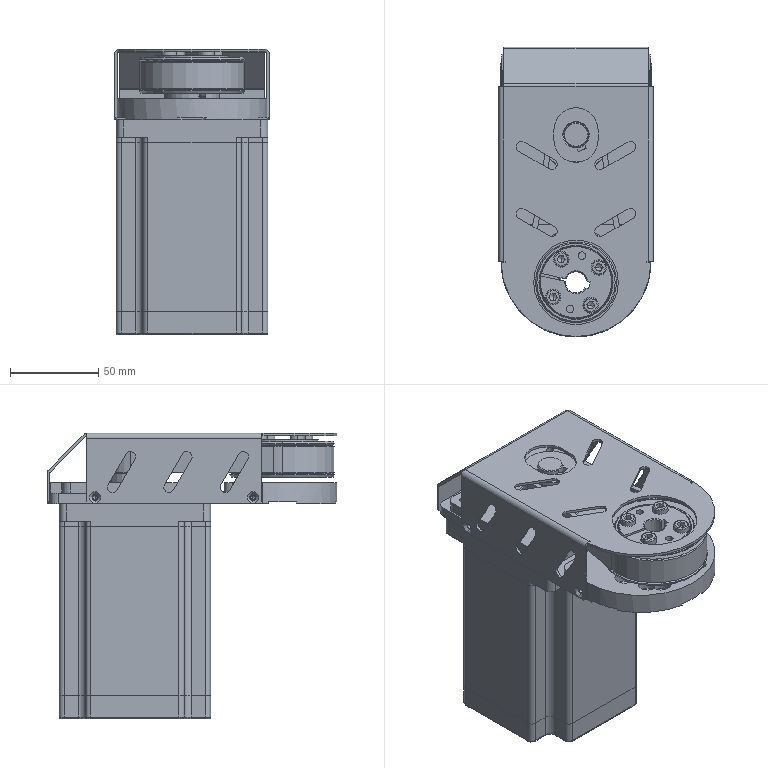Part | STEP file | Copy of CZ020-86 side link 2:1(K60)^K50A-1H20-S(formula driven)-L300-motor left- | 14 solids | 1136 faces | box 88 x 164.5 x 162 mm | volume 999458 mm3 | cylinder 740 | plane 257 | cone 111 | spline 28 | commonest cylinder face diameters 0.6 x219 1.82 x129 56.53 x61 6 x60 4.2 x50 6.5 x34